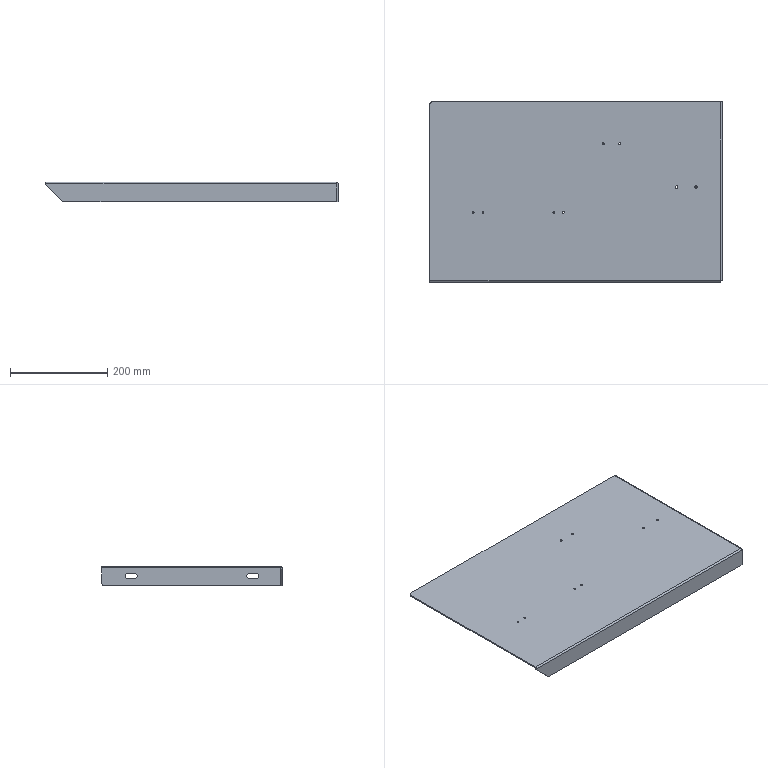Part | NX | features BREP 1 | 1 solid | 49 faces | box 600 x 370 x 40 mm | volume 640302 mm3 | cylinder 26 | plane 21 | spline 2 | commonest cylinder face diameters 3.3 x8 10 x6 4.2 x4 5 x4 1.473 x2 6.473 x2